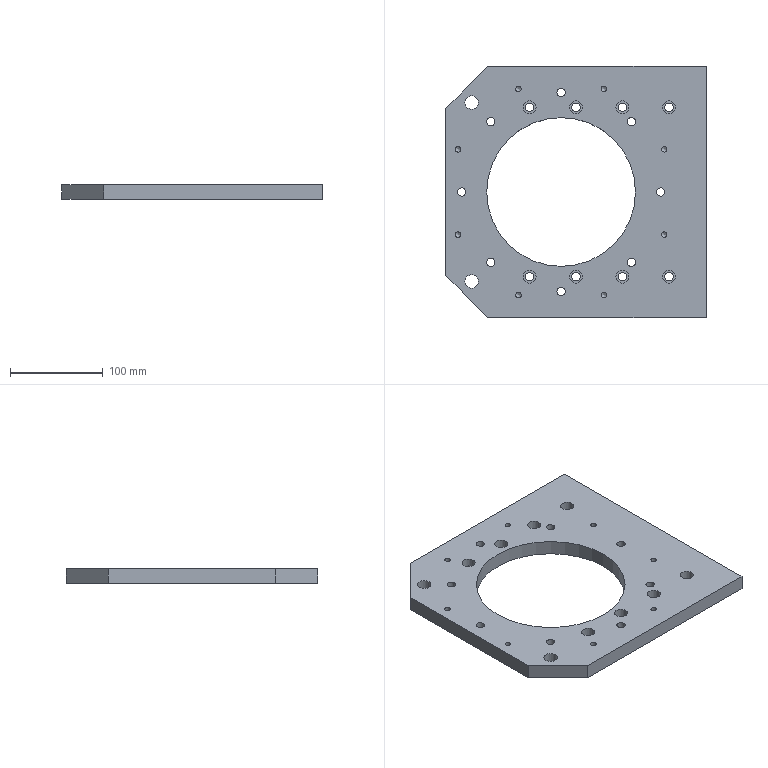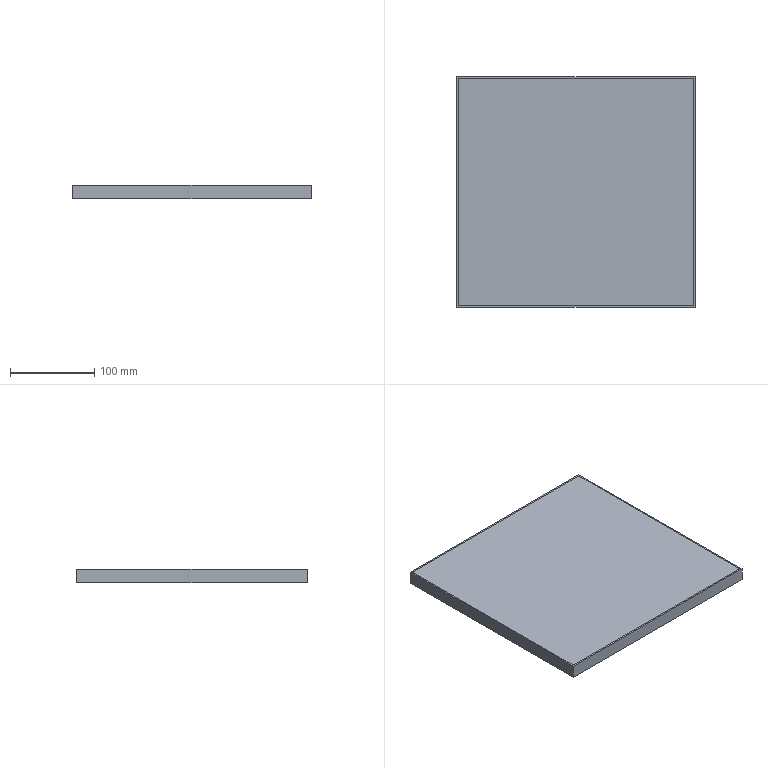CAM job | NX | 3-axis milling, drilling | part box 280 x 270 x 16 mm | stock box 284 x 274 x 16 mm
Tools:
number,name,description,diameter,corner_radius,flute_length,length,flutes
11,ZXZ,Milling Tool-5 Parameters,6.0,0.0,50.0,75.0,2
16,6.0ZT,Drilling Tool,6.0,0.0,35.0,50.0,2
19,9.0ZT,Drilling Tool,9.0,0.0,35.0,50.0,2
14,14.5ZT,Drilling Tool,14.5,0.0,35.0,50.0,2
10,D10,Milling Tool-5 Parameters,10.0,0.0,50.0,75.0,2
9,D10JING,Milling Tool-5 Parameters,10.0,0.0,50.0,75.0,2
6,D6,Milling Tool-5 Parameters,6.0,0.0,50.0,75.0,2
7,D6A45,Milling Tool-5 Parameters,6.0,0.0,3.0,3.0,2
Operations:
program,operation,operation_type,tool,method,geometry_group,spindle_rpm,surface_speed,feed_per_tooth,feed_cut,feed_plunge,cut_length_mm,path_length_mm,cut_time_min,machine_time_min
1压左右,DRILLING,Operation,ZXZ,METHOD,A,3000.0,56.0,0.0417,250.0,0.0,108.0,1458.38,0.432,0.567
1压左右,DRILLING_COPY,Operation,6.0ZT,METHOD,A,2000.0,37.0,0.045,180.0,0.0,118.421,1061.092,0.6579,0.7522
1压左右,DRILLING_COPY_COPY,Operation,9.0ZT,METHOD,A,1000.0,28.0,0.09,180.0,0.0,363.262,1642.575,2.018,2.146
1压左右,DRILLING_COPY_COPY_COPY_COPY,Operation,14.5ZT,METHOD,A,800.0,36.0,0.1125,180.0,0.0,48.712,452.781,0.2706,0.311
1压左右,HOLE_MILLING,CylinderMilling,D10,METHOD,A,3200.0,100.0,0.3438,2200.0,100.0,4492.572,6322.572,2.042,2.225
1压左右,ZLEVEL_PROFILE,ZLevelMilling,D10,METHOD,A,2200.0,69.0,0.5,2200.0,100.0,36895.271,37570.177,16.771,16.838
1压左右,ZLEVEL_PROFILE_COPY_1,ZLevelMilling,D10,METHOD,A,2200.0,69.0,0.5,2200.0,100.0,34461.474,34634.325,15.664,15.682
1压左右,ZLEVEL_PROFILE_COPY,ZLevelMilling,D10JING,METHOD,A,5000.0,157.0,0.12,1200.0,100.0,484.596,1158.934,0.4038,0.4713
1压左右,ZLEVEL_PROFILE_COPY_COPY_1,ZLevelMilling,D6,METHOD,A,5000.0,157.0,0.12,1200.0,100.0,490.349,676.149,0.4086,0.4272
1压左右,ZLEVEL_PROFILE_COPY_COPY,ZLevelMilling,D6A45,METHOD,A,7500.0,141.0,0.08,1200.0,100.0,1893.542,11059.481,1.578,2.494
2压前后,ZLEVEL_PROFILE_COPY_1_1,ZLevelMilling,D10,METHOD,A,2200.0,69.0,0.5,2200.0,100.0,48250.435,48804.166,21.932,21.987
2压前后,ZLEVEL_PROFILE_COPY_COPY_1_1,ZLevelMilling,D10JING,METHOD,A,5000.0,157.0,0.12,1200.0,100.0,639.729,1200.665,0.5331,0.5892
2压前后,ZLEVEL_PROFILE_COPY_COPY_COPY,ZLevelMilling,D6A45,METHOD,A,7500.0,141.0,0.08,1200.0,100.0,623.55,1114.041,0.5196,0.5687
2夹着做,HOLE_MILLING_COPY,CylinderMilling,D10,METHOD,B,3200.0,100.0,0.3438,2200.0,100.0,4492.572,6253.831,2.042,2.218
2夹着做,ZLEVEL_PROFILE_COPY_COPY_COPY_1,ZLevelMilling,D6A45,METHOD,B,7500.0,141.0,0.08,1200.0,100.0,2311.445,7691.995,1.926,2.464